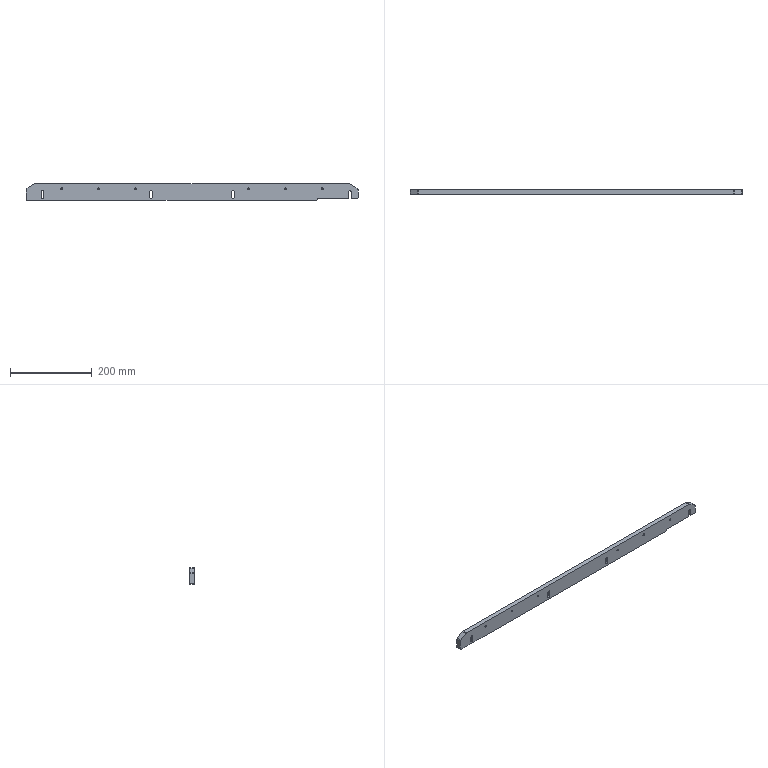CAM job | NX | 3+2 milling, drilling | part box 810 x 12 x 40 mm | stock box 815 x 15 x 45 mm
Tools:
number,name,description,diameter,corner_radius,flute_length,length,flutes
4,D4,平底铣刀-粗,4.0,0.0,25.0,75.0,2
6,D6,平底铣刀-粗,6.0,0.0,25.0,75.0,2
9,D10,平底铣刀-粗,10.0,0.0,35.0,75.0,2
17,D3-J,平底铣刀-精,3.0,0.0,50.0,75.0,2
7,D6-J,平底铣刀-精,6.0,0.0,25.0,75.0,2
1,D80R0.8_FLYCUTTER,圆鼻刀-粗,80.0,0.8,50.0,75.0,2
1,D80R0.8_FLYCUTTER-J,圆鼻刀-精,80.0,0.8,50.0,75.0,2
2,D6_CHAMFERMILL,倒角刀,6.0,0.0,3.0,25.0,2
19,M6X1.0,丝锥,5.0,0.0,35.0,50.0,2
15,ZT5,钻头,5.0,0.0,35.0,50.0,2
Operations:
program,operation,operation_type,tool,method,geometry_group,spindle_rpm,surface_speed,feed_per_tooth,feed_cut,feed_plunge,cut_length_mm,path_length_mm,cut_time_min,machine_time_min
B,BOTTOMWALL_FACEMILL_ONECUT_ROUGH_COPY,VolumeBased25DMillingOperation,D80R0.8_FLYCUTTER,LAYERROUGH-DEPTHK-STEPG,W-B,2800.0,703.696,0.5357,3000.0,100.0,5509.537,10184.167,1.837,2.304
B,BOTTOMWALL_FACEMILL_ONECUT_FINISH_COPY,VolumeBased25DMillingOperation,D80R0.8_FLYCUTTER-J,SIDEFINISH-DEPTHK-STEPG,W-B,4000.0,1005.28,0.125,1000.0,100.0,918.06,954.06,0.9181,0.9217
B,MILLCHAMFER_2,PlanarMilling,D6_CHAMFERMILL,METHOD,W-B,8000.0,150.796,0.0375,600.0,100.0,113.732,1008.228,0.1896,0.279
B,PLANARDEBURR6X45L_COPY,SurfaceContour,D6_CHAMFERMILL,CLIMBCHAMFER-DEPTH0-STEPG,W-B,6500.0,122.519,0.1154,1500.0,100.0,1927.341,3143.919,1.285,1.407
A,TOPFACE,FaceMilling,D80R0.8_FLYCUTTER,SIDEFINISH-DEPTHK-STEPG,W-A,4000.0,1005.31,0.125,1000.0,100.0,904.0,940.0,0.904,0.9076
A,CONTOUR_ROUGH_2,VolumeBased25DMillingOperation,D10,METHOD,W-A,8000.0,251.327,0.3125,5000.0,80.0,29051.08,29101.78,5.81,5.815
A,SPOTDRILL-DEPTH0.8,Operation,D6_CHAMFERMILL,NONE,W-A,8000.0,150.796,0.0312,500.0,90.0,10.8,701.624,0.0216,0.0907
A,THRUHOLE-M6TAPDRILL,Operation,ZT5,NONE,W-A,2800.0,43.982,0.0625,350.0,90.0,123.013,926.05,0.3515,0.4318
A,BLINDSLOT_ROUGH,VolumeBased25DMillingOperation,D6,METHOD,W-A,6000.0,113.097,0.1667,2000.0,100.0,3052.794,3648.895,1.526,1.586
A,THRUSLOT_ROUGH_1,VolumeBased25DMillingOperation,D4,METHOD,W-A,6000.0,75.398,0.1,1200.0,100.0,2275.434,2912.336,1.896,1.96
A,SLOT_FINISH_3,VolumeBased25DMillingOperation,D3-J,METHOD,W-A,6000.0,56.549,0.0667,800.0,100.0,225.228,900.532,0.2815,0.3491
A,CONTOUR_SIDE,ZLevelMilling,D3-J,METHOD,W-A,9000.0,84.823,0.1389,2500.0,80.0,1193.122,1374.826,0.4774,0.4956
A,SELECTBODYONLY,SurfaceContour,D6_CHAMFERMILL,METHOD,W-A,8000.0,150.796,0.1875,3000.0,100.0,1909.611,2612.019,0.6365,0.7068
A,MILLCHAMFER_1,PlanarMilling,D6_CHAMFERMILL,METHOD,W-A,8000.0,150.796,0.0312,500.0,100.0,119.629,991.616,0.2393,0.3265
A,THRUHOLE-TAPM6,Operation,M6X1.0,METHOD,W-A,500.0,7.854,0.001,1.0,90.0,99.0,878.024,99.0,99.078
A,SLOT_FINISH,VolumeBased25DMillingOperation,D6-J,METHOD,W-A,6000.0,113.0,0.0667,600.0,100.0,251.618,896.02,0.4194,0.4838
A,BOTTOMSIDE_FINISH_3,VolumeBased25DMillingOperation,D6-J,METHOD,W-A,6000.0,113.0,0.2083,1200.0,100.0,47.596,100.196,0.0397,0.0449
A,CONTOUR_SEMIFINISH_2,VolumeBased25DMillingOperation,D6-J,METHOD,W-A,8000.0,251.327,0.0625,1000.0,100.0,1734.293,1797.693,1.734,1.741